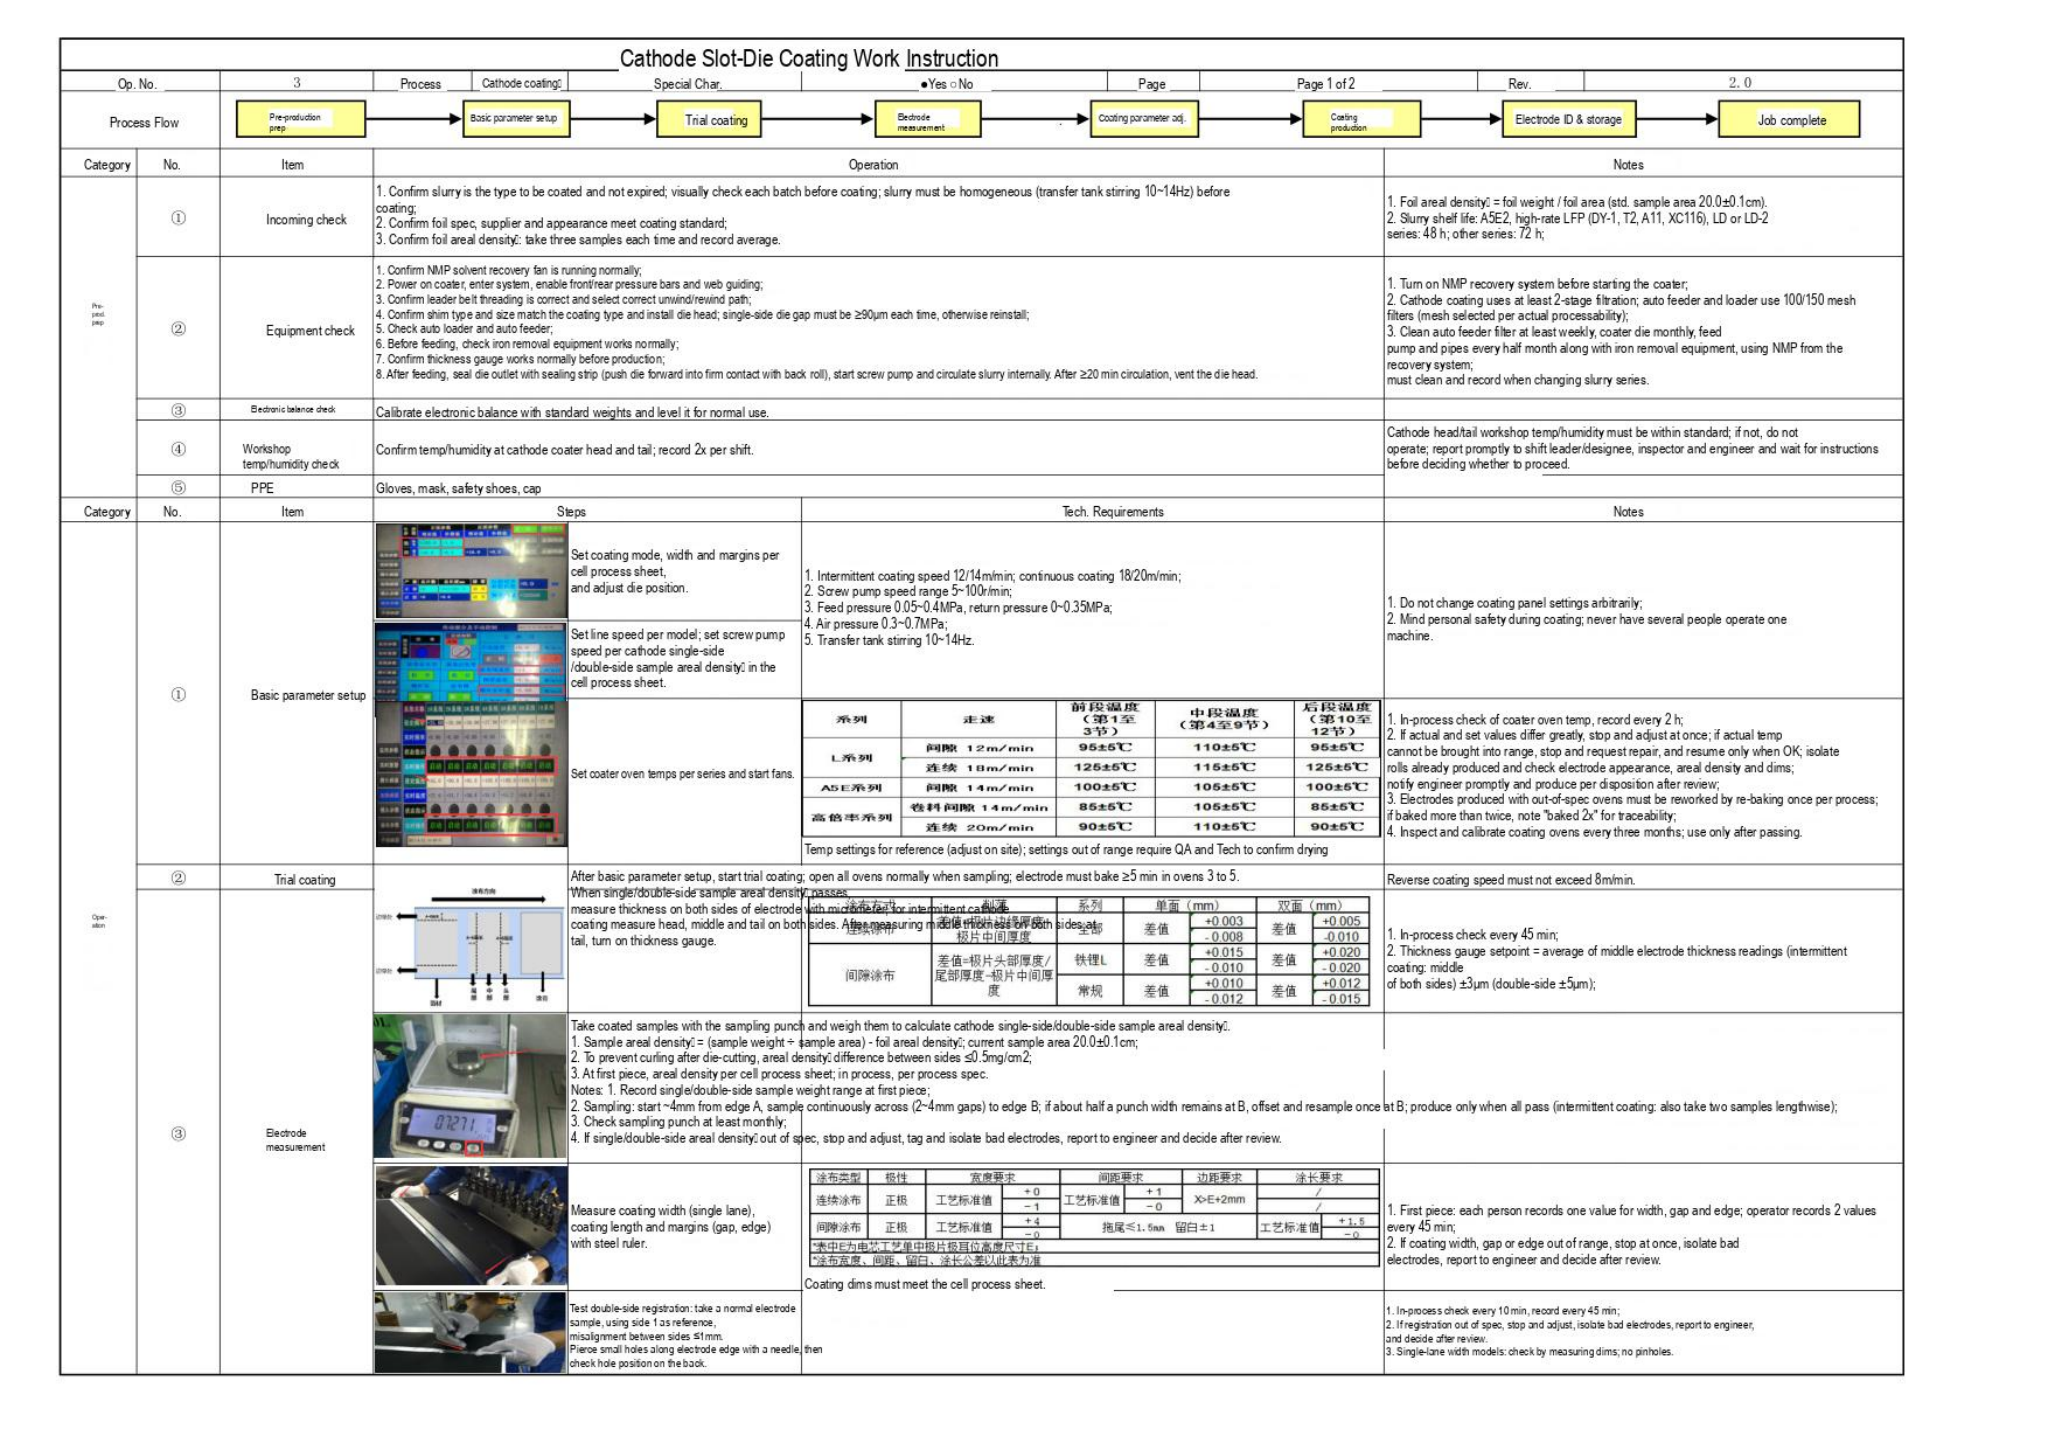# Cathode Slot-Die Coating Work Instruction

| Op. No. | 3 | Process | Cathode coating | Special Char. | ●Yes ○No | Page | Page 1 of 2 | Rev. | 2.0 |
|---|---|---|---|---|---|---|---|---|---|

Process Flow: Pre-production prep → Basic parameter setup → Trial coating → Electrode measurement → Coating parameter adj. → Coating production → Electrode ID & storage → Job complete

| Category | No. | Item | Operation | Notes |
|---|---|---|---|---|
| Pre-prod. prep | ① | Incoming check | 1. Confirm slurry is the type to be coated and not expired; visually check each batch before coating; slurry must be homogeneous (transfer tank stirring 10~14Hz) before coating;<br>2. Confirm foil spec, supplier and appearance meet coating standard;<br>3. Confirm foil areal density: take three samples each time and record average. | 1. Foil areal density = foil weight / foil area (std. sample area 20.0±0.1cm).<br>2. Slurry shelf life: A5E2, high-rate LFP (DY-1, T2, A11, XC116), LD or LD-2 series: 48 h; other series: 72 h; |
| | ② | Equipment check | 1. Confirm NMP solvent recovery fan is running normally;<br>2. Power on coater, enter system, enable front/rear pressure bars and web guiding;<br>3. Confirm leader belt threading is correct and select correct unwind/rewind path;<br>4. Confirm shim type and size match the coating type and install die head; single-side die gap must be ≥90μm each time, otherwise reinstall;<br>5. Check auto loader and auto feeder;<br>6. Before feeding, check iron removal equipment works normally;<br>7. Confirm thickness gauge works normally before production;<br>8. After feeding, seal die outlet with sealing strip (push die forward into firm contact with back roll), start screw pump and circulate slurry internally. After ≥20 min circulation, vent the die head. | 1. Turn on NMP recovery system before starting the coater;<br>2. Cathode coating uses at least 2-stage filtration; auto feeder and loader use 100/150 mesh filters (mesh selected per actual processability);<br>3. Clean auto feeder filter at least weekly, coater die monthly, feed pump and pipes every half month along with iron removal equipment, using NMP from the recovery system;<br>must clean and record when changing slurry series. |
| | ③ | Electronic balance check | Calibrate electronic balance with standard weights and level it for normal use. | |
| | ④ | Workshop temp/humidity check | Confirm temp/humidity at cathode coater head and tail; record 2x per shift. | Cathode head/tail workshop temp/humidity must be within standard; if not, do not operate; report promptly to shift leader/designee, inspector and engineer and wait for instructions before deciding whether to proceed. |
| | ⑤ | PPE | Gloves, mask, safety shoes, cap | |

| Category | No. | Item | Steps | Tech. Requirements | Notes |
|---|---|---|---|---|---|
| Oper-ation | ① | Basic parameter setup | Set coating mode, width and margins per cell process sheet, and adjust die position.<br>Set line speed per model; set screw pump speed per cathode single-side /double-side sample areal density in the cell process sheet. | 1. Intermittent coating speed 12/14m/min; continuous coating 18/20m/min;<br>2. Screw pump speed range 5~100r/min;<br>3. Feed pressure 0.05~0.4MPa, return pressure 0~0.35MPa;<br>4. Air pressure 0.3~0.7MPa;<br>5. Transfer tank stirring 10~14Hz. | 1. Do not change coating panel settings arbitrarily;<br>2. Mind personal safety during coating; never have several people operate one machine. |
| | | | Set coater oven temps per series and start fans. | (see table below)<br>Temp settings for reference (adjust on site); settings out of range require QA and Tech to confirm drying | 1. In-process check of coater oven temp, record every 2 h;<br>2. If actual and set values differ greatly, stop and adjust at once; if actual temp cannot be brought into range, stop and request repair, and resume only when OK; isolate rolls already produced and check electrode appearance, areal density and dims; notify engineer promptly and produce per disposition after review;<br>3. Electrodes produced with out-of-spec ovens must be reworked by re-baking once per process; if baked more than twice, note "baked 2x" for traceability;<br>4. Inspect and calibrate coating ovens every three months; use only after passing. |

| 系列 | 走速 | 前段温度（第1至3节） | 中段温度（第4至9节） | 后段温度（第10至12节） |
|---|---|---|---|---|
| L系列 | 间隙 12m/min | 95±5℃ | 110±5℃ | 95±5℃ |
| | 连续 18m/min | 125±5℃ | 115±5℃ | 125±5℃ |
| A5E系列 | 间隙 14m/min | 100±5℃ | 105±5℃ | 100±5℃ |
| 高倍率系列 | 卷料间隙 14m/min | 85±5℃ | 105±5℃ | 85±5℃ |
| | 连续 20m/min | 90±5℃ | 110±5℃ | 90±5℃ |

| No. | Item | Steps / Tech. Requirements | Notes |
|---|---|---|---|
| ② | Trial coating | After basic parameter setup, start trial coating; open all ovens normally when sampling; electrode must bake ≥5 min in ovens 3 to 5. | Reverse coating speed must not exceed 8m/min. |
| ③ | Electrode measurement | 涂布方向<br>When single/double-side sample areal density passes, measure thickness on both sides of electrode with micrometer; for intermittent coating measure head, middle and tail on both sides. After measuring middle thickness on both sides, at tail, turn on thickness gauge. | 1. In-process check every 45 min;<br>2. Thickness gauge setpoint = average of middle electrode thickness readings (intermittent coating: middle of both sides) ±3μm (double-side ±5μm); |

| 涂布方式 | 偏差 | 系列 | 单面（mm） | | 双面（mm） | |
|---|---|---|---|---|---|---|
| 连续涂布 | 差值=极片边缘厚度-极片中间厚度 | 全部 | 差值 | +0.003 / -0.008 | 差值 | +0.005 / -0.010 |
| 间隙涂布 | 差值=极片头部厚度/尾部厚度-极片中间厚度 | 铁锂L | 差值 | +0.015 / -0.010 | 差值 | +0.020 / -0.020 |
| | | 常规 | 差值 | +0.010 / -0.012 | 差值 | +0.012 / -0.015 |

Take coated samples with the sampling punch and weigh them to calculate cathode single-side/double-side sample areal density.
1. Sample areal density = (sample weight ÷ sample area) - foil areal density; current sample area 20.0±0.1cm;
2. To prevent curling after die-cutting, areal density difference between sides ≤0.5mg/cm2;
3. At first piece, areal density per cell process sheet; in process, per process spec.
Notes: 1. Record single/double-side sample weight range at first piece;
2. Sampling: start ~4mm from edge A, sample continuously across (2~4mm gaps) to edge B; if about half a punch width remains at B, offset and resample once at B; produce only when all pass (intermittent coating: also take two samples lengthwise);
3. Check sampling punch at least monthly;
4. If single/double-side areal density out of spec, stop and adjust, tag and isolate bad electrodes, report to engineer and decide after review.

| Steps | Tech. Requirements | Notes |
|---|---|---|
| Measure coating width (single lane), coating length and margins (gap, edge) with steel ruler. | (see table below)<br>Coating dims must meet the cell process sheet. | 1. First piece: each person records one value for width, gap and edge; operator records 2 values every 45 min;<br>2. If coating width, gap or edge out of range, stop at once, isolate bad electrodes, report to engineer and decide after review. |
| Test double-side registration: take a normal electrode sample, using side 1 as reference, misalignment between sides ≤1mm.<br>Pierce small holes along electrode edge with a needle, then check hole position on the back. | | 1. In-process check every 10 min, record every 45 min;<br>2. If registration out of spec, stop and adjust, isolate bad electrodes, report to engineer, and decide after review.<br>3. Single-lane width models: check by measuring dims; no pinholes. |

| 涂布类型 | 极性 | 宽度要求 | | 间距要求 | | 边距要求 | 涂长要求 | |
|---|---|---|---|---|---|---|---|---|
| 连续涂布 | 正极 | 工艺标准值 | +0 / -1 | 工艺标准值 | +1 / -0 | X>E+2mm | / | |
| 间隙涂布 | 正极 | 工艺标准值 | +4 / -0 | 拖尾≤1.5mm 留白±1 | | | 工艺标准值 | +1.5 / -0 |

*表中E为电芯工艺单中极片极耳位高度尺寸E；
*涂布宽度、间距、留白、涂长公差以此表为准
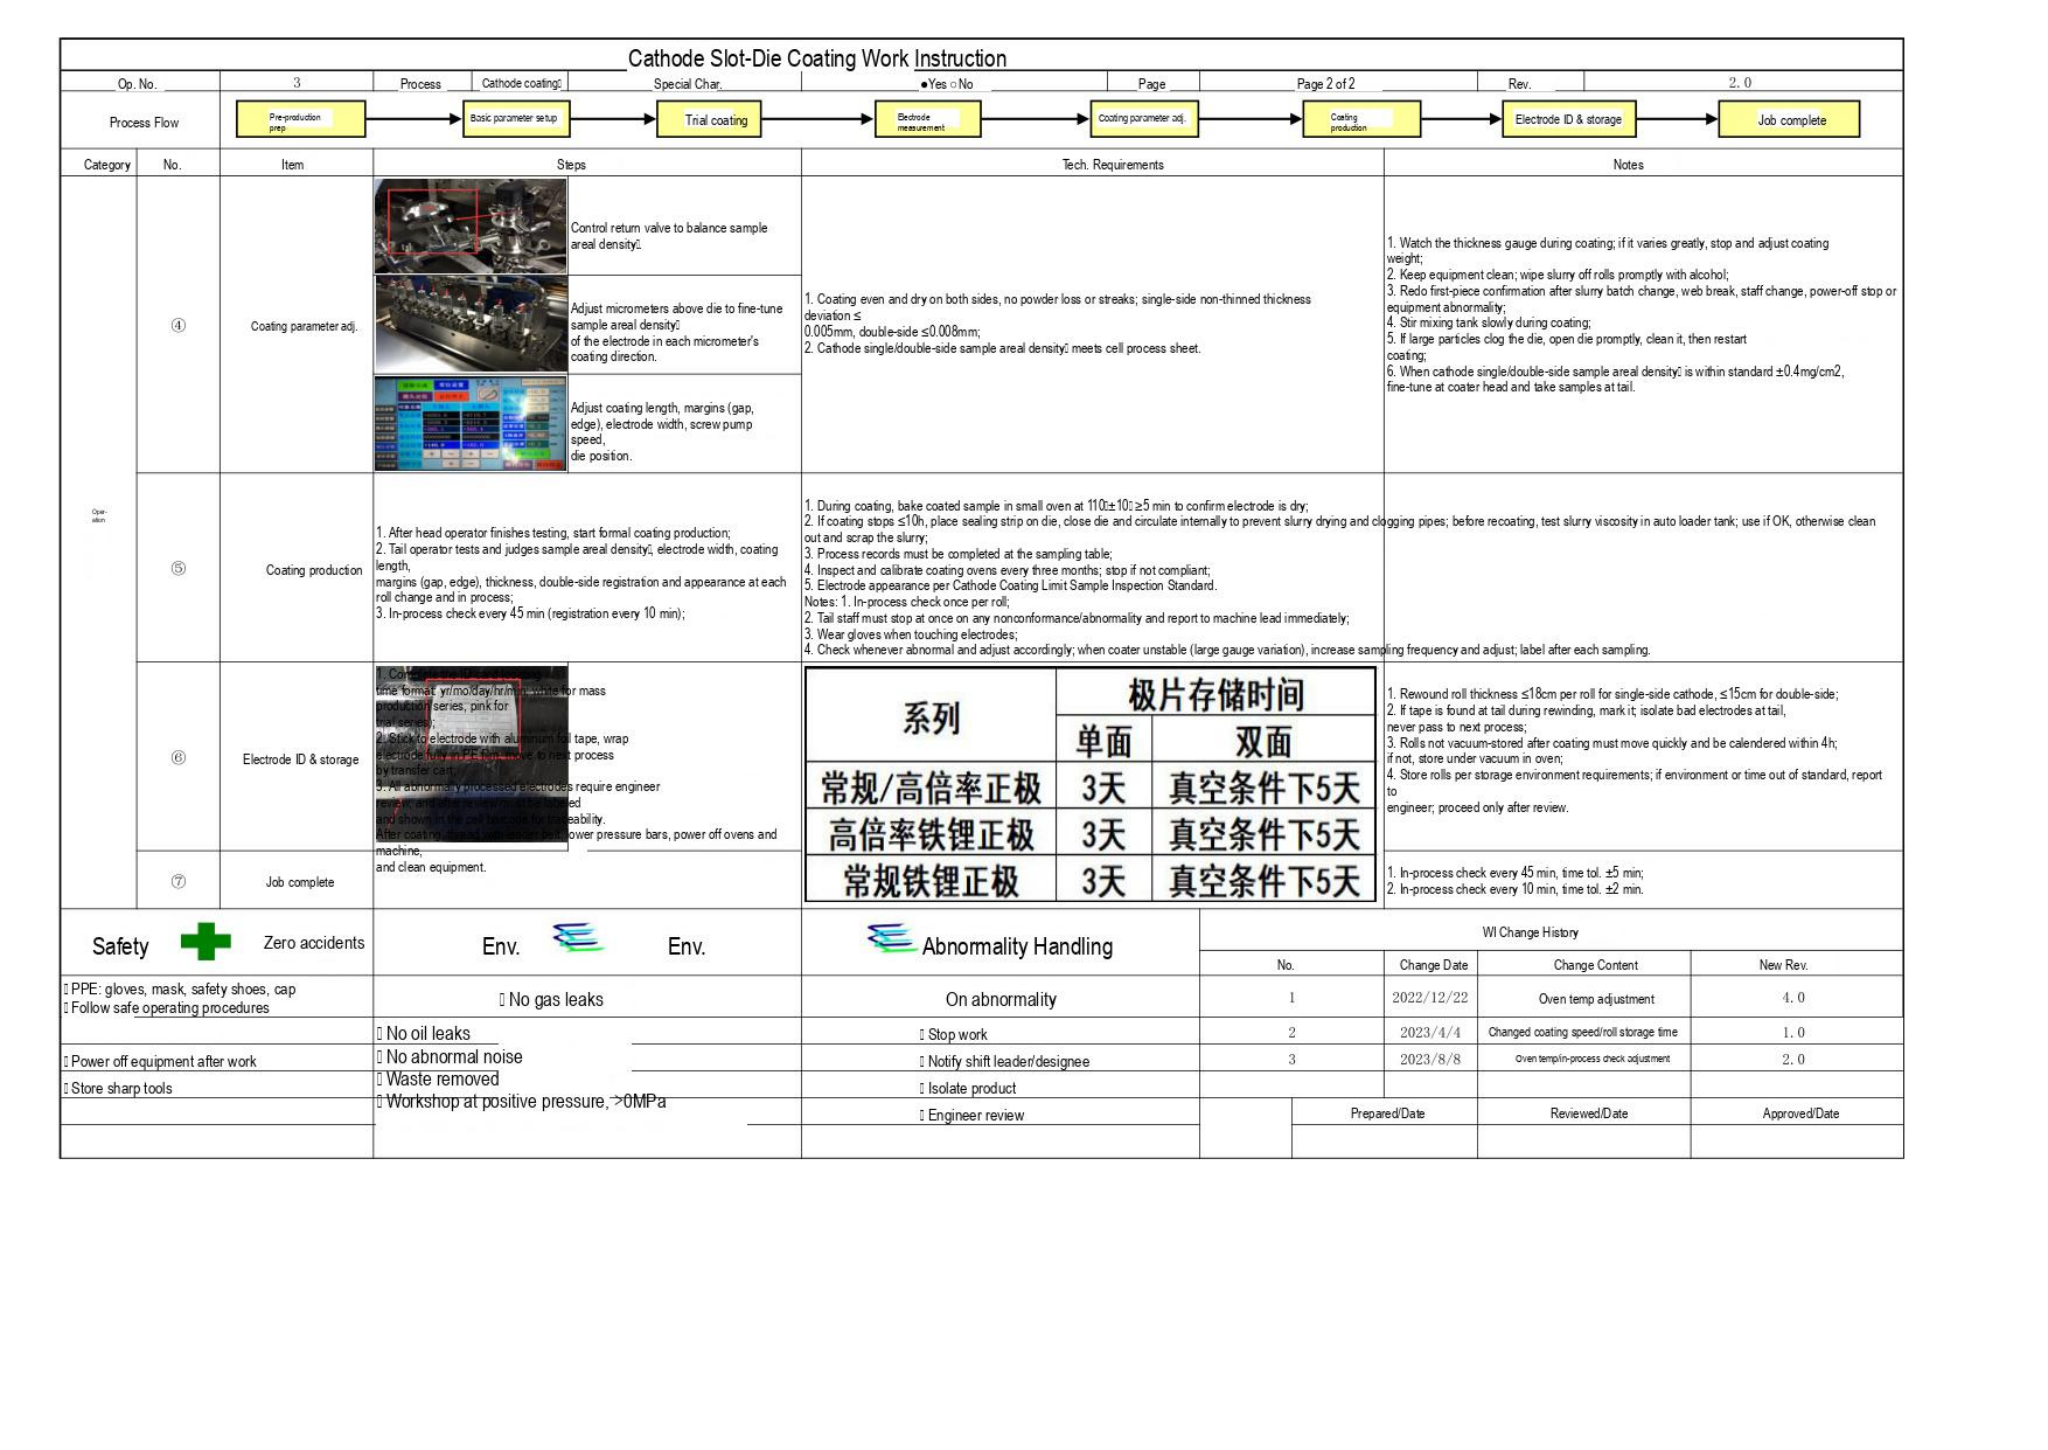# Cathode Slot-Die Coating Work Instruction

| Op. No. | 3 | Process | Cathode coating | Special Char. | ●Yes ○No | Page | Page 2 of 2 | Rev. | 2.0 |
|---|---|---|---|---|---|---|---|---|---|

**Process Flow:** Pre-production prep → Basic parameter setup → Trial coating → Electrode measurement → Coating parameter adj. → Coating production → Electrode ID & storage → Job complete

| Category | No. | Item | Steps | Tech. Requirements | Notes |
|---|---|---|---|---|---|
| Operation | ④ | Coating parameter adj. | Control return valve to balance sample areal density.<br>Adjust micrometers above die to fine-tune sample areal density of the electrode in each micrometer's coating direction.<br>Adjust coating length, margins (gap, edge), electrode width, screw pump speed, die position. | 1. Coating even and dry on both sides, no powder loss or streaks; single-side non-thinned thickness deviation ≤ 0.005mm, double-side ≤0.008mm;<br>2. Cathode single/double-side sample areal density meets cell process sheet. | 1. Watch the thickness gauge during coating; if it varies greatly, stop and adjust coating weight;<br>2. Keep equipment clean; wipe slurry off rolls promptly with alcohol;<br>3. Redo first-piece confirmation after slurry batch change, web break, staff change, power-off stop or equipment abnormality;<br>4. Stir mixing tank slowly during coating;<br>5. If large particles clog the die, open die promptly, clean it, then restart coating;<br>6. When cathode single/double-side sample areal density is within standard ±0.4mg/cm2, fine-tune at coater head and take samples at tail. |
| | ⑤ | Coating production | 1. After head operator finishes testing, start formal coating production;<br>2. Tail operator tests and judges sample areal density, electrode width, coating length, margins (gap, edge), thickness, double-side registration and appearance at each roll change and in process;<br>3. In-process check every 45 min (registration every 10 min); | 1. During coating, bake coated sample in small oven at 110±10 ≥5 min to confirm electrode is dry;<br>2. If coating stops ≤10h, place sealing strip on die, close die and circulate internally to prevent slurry drying and clogging pipes; before recoating, test slurry viscosity in auto loader tank; use if OK, otherwise clean out and scrap the slurry;<br>3. Process records must be completed at the sampling table;<br>4. Inspect and calibrate coating ovens every three months; stop if not compliant;<br>5. Electrode appearance per Cathode Coating Limit Sample Inspection Standard.<br>Notes: 1. In-process check once per roll;<br>2. Tail staff must stop at once on any nonconformance/abnormality and report to machine lead immediately;<br>3. Wear gloves when touching electrodes;<br>4. Check whenever abnormal and adjust accordingly; when coater unstable (large gauge variation), increase sampling frequency and adjust; label after each sampling. | |
| | ⑥ | Electrode ID & storage | 1. Co... time format: yr/mo/day/hr/m... white for mass production series, pink for trial series;<br>2. Stick to electrode with aluminum foil tape, wrap electrode fully in PE film ... to next process by transfer cart;<br>3. All abnormally processed electrodes require engineer review, and ... labeled and shown in the cell ... for traceability.<br>After coating, ... lower pressure bars, power off ovens and machine, and clean equipment. | (see table below) | 1. Rewound roll thickness ≤18cm per roll for single-side cathode, ≤15cm for double-side;<br>2. If tape is found at tail during rewinding, mark it; isolate bad electrodes at tail, never pass to next process;<br>3. Rolls not vacuum-stored after coating must move quickly and be calendered within 4h; if not, store under vacuum in oven;<br>4. Store rolls per storage environment requirements; if environment or time out of standard, report to engineer; proceed only after review. |
| | ⑦ | Job complete | | | 1. In-process check every 45 min, time tol. ±5 min;<br>2. In-process check every 10 min, time tol. ±2 min. |

| 系列 | 极片存储时间 单面 | 极片存储时间 双面 |
|---|---|---|
| 常规/高倍率正极 | 3天 | 真空条件下5天 |
| 高倍率铁锂正极 | 3天 | 真空条件下5天 |
| 常规铁锂正极 | 3天 | 真空条件下5天 |

| Safety — Zero accidents | Env. — Env. | Abnormality Handling |
|---|---|---|
| PPE: gloves, mask, safety shoes, cap<br>Follow safe operating procedures | No gas leaks | On abnormality |
| | No oil leaks | Stop work |
| Power off equipment after work | No abnormal noise | Notify shift leader/designee |
| Store sharp tools | Waste removed | Isolate product |
| | Workshop at positive pressure, >0MPa | Engineer review |

**WI Change History**

| No. | Change Date | Change Content | New Rev. |
|---|---|---|---|
| 1 | 2022/12/22 | Oven temp adjustment | 4.0 |
| 2 | 2023/4/4 | Changed coating speed/roll storage time | 1.0 |
| 3 | 2023/8/8 | Oven temp/in-process check adjustment | 2.0 |

| Prepared/Date | Reviewed/Date | Approved/Date |
|---|---|---|
| | | |